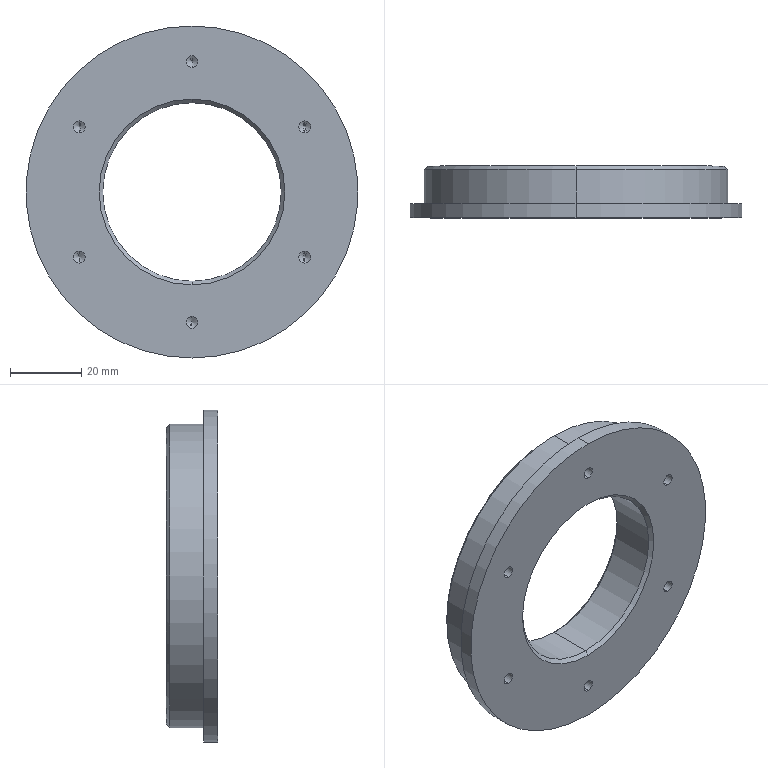Part | SolidWorks | features Chamfer 1, HoleWzd 1, Revolution 1 | 1 solid | 39 faces | box 93 x 14.5 x 93 mm | volume 57472 mm3 | cone 18 | cylinder 18 | plane 3 | commonest cylinder face diameters 3.3 x12 50 x2 85 x2 93 x2
STEP:
#1=CARTESIAN_POINT('',(0.,14.5,41.5));
#2=VERTEX_POINT('',#1);
#3=CARTESIAN_POINT('',(0.,14.5,-41.5));
#4=VERTEX_POINT('',#3);
#5=CARTESIAN_POINT('',(0.,14.5,0.));
#6=DIRECTION('',(0.,1.,0.));
#7=DIRECTION('',(0.,0.,1.));
#8=AXIS2_PLACEMENT_3D('',#5,#6,#7);
#9=CIRCLE('',#8,41.5);
#10=EDGE_CURVE('',#2,#4,#9,.T.);
#11=ORIENTED_EDGE('',*,*,#10,.F.);
#12=CARTESIAN_POINT('',(0.,13.5,42.5));
#13=VERTEX_POINT('',#12);
#14=CARTESIAN_POINT('',(0.,13.5,42.5));
#15=DIRECTION('',(0.,-0.7071,0.7071));
#16=VECTOR('',#15,1000.);
#17=LINE('',#14,#16);
#18=EDGE_CURVE('',#2,#13,#17,.T.);
#19=ORIENTED_EDGE('',*,*,#18,.T.);
#20=CARTESIAN_POINT('',(0.,13.5,-42.5));
#21=VERTEX_POINT('',#20);
#22=CARTESIAN_POINT('',(0.,13.5,0.));
#23=DIRECTION('',(0.,-1.,0.));
#24=DIRECTION('',(0.,0.,1.));
#25=AXIS2_PLACEMENT_3D('',#22,#23,#24);
#26=CIRCLE('',#25,42.5);
#27=EDGE_CURVE('',#21,#13,#26,.T.);
#28=ORIENTED_EDGE('',*,*,#27,.F.);
#29=CARTESIAN_POINT('',(0.,13.5,-42.5));
#30=DIRECTION('',(0.,-0.7071,-0.7071));
#31=VECTOR('',#30,1000.);
#32=LINE('',#29,#31);
#33=EDGE_CURVE('',#4,#21,#32,.T.);
#34=ORIENTED_EDGE('',*,*,#33,.F.);
#35=EDGE_LOOP('',(#11,#19,#28,#34));
#36=FACE_OUTER_BOUND('',#35,.T.);
#37=CARTESIAN_POINT('',(0.,13.5,0.));
#38=DIRECTION('',(0.,-1.,0.));
#39=DIRECTION('',(0.,0.,-1.));
#40=AXIS2_PLACEMENT_3D('',#37,#38,#39);
#41=CONICAL_SURFACE('',#40,42.5,0.7854);
#42=ADVANCED_FACE('',(#36),#41,.T.);
#43=CARTESIAN_POINT('',(0.,13.5,-25.));
#44=VERTEX_POINT('',#43);
#45=CARTESIAN_POINT('',(0.,13.5,25.));
#46=VERTEX_POINT('',#45);
#47=CARTESIAN_POINT('',(0.,13.5,0.));
#48=DIRECTION('',(0.,1.,0.));
#49=DIRECTION('',(0.,0.,1.));
#50=AXIS2_PLACEMENT_3D('',#47,#48,#49);
#51=CIRCLE('',#50,25.);
#52=EDGE_CURVE('',#44,#46,#51,.T.);
#53=ORIENTED_EDGE('',*,*,#52,.F.);
#54=CARTESIAN_POINT('',(0.,14.5,-26.));
#55=VERTEX_POINT('',#54);
#56=CARTESIAN_POINT('',(0.,14.5,-26.));
#57=DIRECTION('',(0.,0.7071,-0.7071));
#58=VECTOR('',#57,1000.);
#59=LINE('',#56,#58);
#60=EDGE_CURVE('',#44,#55,#59,.T.);
#61=ORIENTED_EDGE('',*,*,#60,.T.);
#62=CARTESIAN_POINT('',(0.,14.5,26.));
#63=VERTEX_POINT('',#62);
#64=CARTESIAN_POINT('',(0.,14.5,0.));
#65=DIRECTION('',(0.,-1.,0.));
#66=DIRECTION('',(0.,0.,1.));
#67=AXIS2_PLACEMENT_3D('',#64,#65,#66);
#68=CIRCLE('',#67,26.);
#69=EDGE_CURVE('',#63,#55,#68,.T.);
#70=ORIENTED_EDGE('',*,*,#69,.F.);
#71=CARTESIAN_POINT('',(0.,14.5,26.));
#72=DIRECTION('',(0.,0.7071,0.7071));
#73=VECTOR('',#72,1000.);
#74=LINE('',#71,#73);
#75=EDGE_CURVE('',#46,#63,#74,.T.);
#76=ORIENTED_EDGE('',*,*,#75,.F.);
#77=EDGE_LOOP('',(#53,#61,#70,#76));
#78=FACE_OUTER_BOUND('',#77,.T.);
#79=CARTESIAN_POINT('',(0.,14.5,0.));
#80=DIRECTION('',(0.,1.,0.));
#81=DIRECTION('',(0.,0.,1.));
#82=AXIS2_PLACEMENT_3D('',#79,#80,#81);
#83=CONICAL_SURFACE('',#82,26.,0.7854);
#84=ADVANCED_FACE('',(#78),#83,.F.);
#85=CARTESIAN_POINT('',(0.,1.,25.));
#86=VERTEX_POINT('',#85);
#87=CARTESIAN_POINT('',(0.,1.,-25.));
#88=VERTEX_POINT('',#87);
#89=CARTESIAN_POINT('',(0.,1.,0.));
#90=DIRECTION('',(0.,-1.,0.));
#91=DIRECTION('',(0.,0.,-1.));
#92=AXIS2_PLACEMENT_3D('',#89,#90,#91);
#93=CIRCLE('',#92,25.);
#94=EDGE_CURVE('',#86,#88,#93,.T.);
#95=ORIENTED_EDGE('',*,*,#94,.F.);
#96=CARTESIAN_POINT('',(0.,0.,26.));
#97=VERTEX_POINT('',#96);
#98=CARTESIAN_POINT('',(0.,1.,25.));
#99=DIRECTION('',(0.,-0.7071,0.7071));
#100=VECTOR('',#99,1000.);
#101=LINE('',#98,#100);
#102=EDGE_CURVE('',#86,#97,#101,.T.);
#103=ORIENTED_EDGE('',*,*,#102,.T.);
#104=CARTESIAN_POINT('',(0.,0.,-26.));
#105=VERTEX_POINT('',#104);
#106=CARTESIAN_POINT('',(0.,0.,0.));
#107=DIRECTION('',(0.,1.,0.));
#108=DIRECTION('',(0.,0.,-1.));
#109=AXIS2_PLACEMENT_3D('',#106,#107,#108);
#110=CIRCLE('',#109,26.);
#111=EDGE_CURVE('',#105,#97,#110,.T.);
#112=ORIENTED_EDGE('',*,*,#111,.F.);
#113=CARTESIAN_POINT('',(0.,1.,-25.));
#114=DIRECTION('',(0.,-0.7071,-0.7071));
#115=VECTOR('',#114,1000.);
#116=LINE('',#113,#115);
#117=EDGE_CURVE('',#88,#105,#116,.T.);
#118=ORIENTED_EDGE('',*,*,#117,.F.);
#119=EDGE_LOOP('',(#95,#103,#112,#118));
#120=FACE_OUTER_BOUND('',#119,.T.);
#121=CARTESIAN_POINT('',(0.,1.,0.));
#122=DIRECTION('',(0.,-1.,0.));
#123=DIRECTION('',(0.,0.,-1.));
#124=AXIS2_PLACEMENT_3D('',#121,#122,#123);
#125=CONICAL_SURFACE('',#124,25.,0.7854);
#126=ADVANCED_FACE('',(#120),#125,.F.);
#127=CARTESIAN_POINT('',(0.,9.8,38.15));
#128=VERTEX_POINT('',#127);
#129=CARTESIAN_POINT('',(0.,9.8,34.85));
#130=VERTEX_POINT('',#129);
#131=CARTESIAN_POINT('',(0.,9.8,36.5));
#132=DIRECTION('',(0.,-1.,0.));
#133=DIRECTION('',(0.,0.,-1.));
#134=AXIS2_PLACEMENT_3D('',#131,#132,#133);
#135=CIRCLE('',#134,1.65);
#136=EDGE_CURVE('',#128,#130,#135,.T.);
#137=ORIENTED_EDGE('',*,*,#136,.F.);
#138=CARTESIAN_POINT('',(0.,0.,38.15));
#139=VERTEX_POINT('',#138);
#140=CARTESIAN_POINT('',(0.,0.,38.15));
#141=DIRECTION('',(0.,-1.,0.));
#142=VECTOR('',#141,1000.);
#143=LINE('',#140,#142);
#144=EDGE_CURVE('',#128,#139,#143,.T.);
#145=ORIENTED_EDGE('',*,*,#144,.T.);
#146=CARTESIAN_POINT('',(0.,0.,34.85));
#147=VERTEX_POINT('',#146);
#148=CARTESIAN_POINT('',(0.,0.,36.5));
#149=DIRECTION('',(0.,-1.,0.));
#150=DIRECTION('',(0.,0.,-1.));
#151=AXIS2_PLACEMENT_3D('',#148,#149,#150);
#152=CIRCLE('',#151,1.65);
#153=EDGE_CURVE('',#139,#147,#152,.T.);
#154=ORIENTED_EDGE('',*,*,#153,.T.);
#155=CARTESIAN_POINT('',(0.,0.,34.85));
#156=DIRECTION('',(0.,-1.,0.));
#157=VECTOR('',#156,1000.);
#158=LINE('',#155,#157);
#159=EDGE_CURVE('',#130,#147,#158,.T.);
#160=ORIENTED_EDGE('',*,*,#159,.F.);
#161=EDGE_LOOP('',(#137,#145,#154,#160));
#162=FACE_OUTER_BOUND('',#161,.T.);
#163=CARTESIAN_POINT('',(0.,0.,36.5));
#164=DIRECTION('',(0.,-1.,0.));
#165=DIRECTION('',(0.,0.,-1.));
#166=AXIS2_PLACEMENT_3D('',#163,#164,#165);
#167=CYLINDRICAL_SURFACE('',#166,1.65);
#168=ADVANCED_FACE('',(#162),#167,.F.);
#169=CARTESIAN_POINT('',(0.,10.791,36.5));
#170=VERTEX_POINT('',#169);
#171=CARTESIAN_POINT('',(0.,9.8,34.85));
#172=DIRECTION('',(0.,-0.515,-0.8572));
#173=VECTOR('',#172,1000.);
#174=LINE('',#171,#173);
#175=EDGE_CURVE('',#170,#130,#174,.T.);
#176=ORIENTED_EDGE('',*,*,#175,.F.);
#177=CARTESIAN_POINT('',(0.,9.8,38.15));
#178=DIRECTION('',(0.,-0.515,0.8572));
#179=VECTOR('',#178,1000.);
#180=LINE('',#177,#179);
#181=EDGE_CURVE('',#170,#128,#180,.T.);
#182=ORIENTED_EDGE('',*,*,#181,.T.);
#183=ORIENTED_EDGE('',*,*,#136,.T.);
#184=EDGE_LOOP('',(#176,#182,#183));
#185=FACE_OUTER_BOUND('',#184,.T.);
#186=CARTESIAN_POINT('',(0.,9.8,36.5));
#187=DIRECTION('',(0.,-1.,0.));
#188=DIRECTION('',(0.,0.,-1.));
#189=AXIS2_PLACEMENT_3D('',#186,#187,#188);
#190=CONICAL_SURFACE('',#189,1.65,1.03);
#191=ADVANCED_FACE('',(#185),#190,.F.);
#192=CARTESIAN_POINT('',(31.61,9.8,19.9));
#193=VERTEX_POINT('',#192);
#194=CARTESIAN_POINT('',(31.61,9.8,16.6));
#195=VERTEX_POINT('',#194);
#196=CARTESIAN_POINT('',(31.61,9.8,18.25));
#197=DIRECTION('',(0.,-1.,0.));
#198=DIRECTION('',(0.,0.,-1.));
#199=AXIS2_PLACEMENT_3D('',#196,#197,#198);
#200=CIRCLE('',#199,1.65);
#201=EDGE_CURVE('',#193,#195,#200,.T.);
#202=ORIENTED_EDGE('',*,*,#201,.F.);
#203=CARTESIAN_POINT('',(31.61,0.,19.9));
#204=VERTEX_POINT('',#203);
#205=CARTESIAN_POINT('',(31.61,0.,19.9));
#206=DIRECTION('',(0.,-1.,0.));
#207=VECTOR('',#206,1000.);
#208=LINE('',#205,#207);
#209=EDGE_CURVE('',#193,#204,#208,.T.);
#210=ORIENTED_EDGE('',*,*,#209,.T.);
#211=CARTESIAN_POINT('',(31.61,0.,16.6));
#212=VERTEX_POINT('',#211);
#213=CARTESIAN_POINT('',(31.61,0.,18.25));
#214=DIRECTION('',(0.,-1.,0.));
#215=DIRECTION('',(0.,0.,-1.));
#216=AXIS2_PLACEMENT_3D('',#213,#214,#215);
#217=CIRCLE('',#216,1.65);
#218=EDGE_CURVE('',#204,#212,#217,.T.);
#219=ORIENTED_EDGE('',*,*,#218,.T.);
#220=CARTESIAN_POINT('',(31.61,0.,16.6));
#221=DIRECTION('',(0.,-1.,0.));
#222=VECTOR('',#221,1000.);
#223=LINE('',#220,#222);
#224=EDGE_CURVE('',#195,#212,#223,.T.);
#225=ORIENTED_EDGE('',*,*,#224,.F.);
#226=EDGE_LOOP('',(#202,#210,#219,#225));
#227=FACE_OUTER_BOUND('',#226,.T.);
#228=CARTESIAN_POINT('',(31.61,0.,18.25));
#229=DIRECTION('',(0.,-1.,0.));
#230=DIRECTION('',(0.,0.,-1.));
#231=AXIS2_PLACEMENT_3D('',#228,#229,#230);
#232=CYLINDRICAL_SURFACE('',#231,1.65);
#233=ADVANCED_FACE('',(#227),#232,.F.);
#234=CARTESIAN_POINT('',(31.61,10.791,18.25));
#235=VERTEX_POINT('',#234);
#236=CARTESIAN_POINT('',(31.61,9.8,16.6));
#237=DIRECTION('',(0.,-0.515,-0.8572));
#238=VECTOR('',#237,1000.);
#239=LINE('',#236,#238);
#240=EDGE_CURVE('',#235,#195,#239,.T.);
#241=ORIENTED_EDGE('',*,*,#240,.F.);
#242=CARTESIAN_POINT('',(31.61,9.8,19.9));
#243=DIRECTION('',(0.,-0.515,0.8572));
#244=VECTOR('',#243,1000.);
#245=LINE('',#242,#244);
#246=EDGE_CURVE('',#235,#193,#245,.T.);
#247=ORIENTED_EDGE('',*,*,#246,.T.);
#248=ORIENTED_EDGE('',*,*,#201,.T.);
#249=EDGE_LOOP('',(#241,#247,#248));
#250=FACE_OUTER_BOUND('',#249,.T.);
#251=CARTESIAN_POINT('',(31.61,9.8,18.25));
#252=DIRECTION('',(0.,-1.,0.));
#253=DIRECTION('',(0.,0.,-1.));
#254=AXIS2_PLACEMENT_3D('',#251,#252,#253);
#255=CONICAL_SURFACE('',#254,1.65,1.03);
#256=ADVANCED_FACE('',(#250),#255,.F.);
#257=CARTESIAN_POINT('',(31.61,9.8,-16.6));
#258=VERTEX_POINT('',#257);
#259=CARTESIAN_POINT('',(31.61,9.8,-19.9));
#260=VERTEX_POINT('',#259);
#261=CARTESIAN_POINT('',(31.61,9.8,-18.25));
#262=DIRECTION('',(0.,-1.,0.));
#263=DIRECTION('',(0.,0.,-1.));
#264=AXIS2_PLACEMENT_3D('',#261,#262,#263);
#265=CIRCLE('',#264,1.65);
#266=EDGE_CURVE('',#258,#260,#265,.T.);
#267=ORIENTED_EDGE('',*,*,#266,.F.);
#268=CARTESIAN_POINT('',(31.61,0.,-16.6));
#269=VERTEX_POINT('',#268);
#270=CARTESIAN_POINT('',(31.61,0.,-16.6));
#271=DIRECTION('',(0.,-1.,0.));
#272=VECTOR('',#271,1000.);
#273=LINE('',#270,#272);
#274=EDGE_CURVE('',#258,#269,#273,.T.);
#275=ORIENTED_EDGE('',*,*,#274,.T.);
#276=CARTESIAN_POINT('',(31.61,0.,-19.9));
#277=VERTEX_POINT('',#276);
#278=CARTESIAN_POINT('',(31.61,0.,-18.25));
#279=DIRECTION('',(0.,-1.,0.));
#280=DIRECTION('',(0.,0.,-1.));
#281=AXIS2_PLACEMENT_3D('',#278,#279,#280);
#282=CIRCLE('',#281,1.65);
#283=EDGE_CURVE('',#269,#277,#282,.T.);
#284=ORIENTED_EDGE('',*,*,#283,.T.);
#285=CARTESIAN_POINT('',(31.61,0.,-19.9));
#286=DIRECTION('',(0.,-1.,0.));
#287=VECTOR('',#286,1000.);
#288=LINE('',#285,#287);
#289=EDGE_CURVE('',#260,#277,#288,.T.);
#290=ORIENTED_EDGE('',*,*,#289,.F.);
#291=EDGE_LOOP('',(#267,#275,#284,#290));
#292=FACE_OUTER_BOUND('',#291,.T.);
#293=CARTESIAN_POINT('',(31.61,0.,-18.25));
#294=DIRECTION('',(0.,-1.,0.));
#295=DIRECTION('',(0.,0.,-1.));
#296=AXIS2_PLACEMENT_3D('',#293,#294,#295);
#297=CYLINDRICAL_SURFACE('',#296,1.65);
#298=ADVANCED_FACE('',(#292),#297,.F.);
#299=CARTESIAN_POINT('',(31.61,10.791,-18.25));
#300=VERTEX_POINT('',#299);
#301=CARTESIAN_POINT('',(31.61,9.8,-19.9));
#302=DIRECTION('',(0.,-0.515,-0.8572));
#303=VECTOR('',#302,1000.);
#304=LINE('',#301,#303);
#305=EDGE_CURVE('',#300,#260,#304,.T.);
#306=ORIENTED_EDGE('',*,*,#305,.F.);
#307=CARTESIAN_POINT('',(31.61,9.8,-16.6));
#308=DIRECTION('',(0.,-0.515,0.8572));
#309=VECTOR('',#308,1000.);
#310=LINE('',#307,#309);
#311=EDGE_CURVE('',#300,#258,#310,.T.);
#312=ORIENTED_EDGE('',*,*,#311,.T.);
#313=ORIENTED_EDGE('',*,*,#266,.T.);
#314=EDGE_LOOP('',(#306,#312,#313));
#315=FACE_OUTER_BOUND('',#314,.T.);
#316=CARTESIAN_POINT('',(31.61,9.8,-18.25));
#317=DIRECTION('',(0.,-1.,0.));
#318=DIRECTION('',(0.,0.,-1.));
#319=AXIS2_PLACEMENT_3D('',#316,#317,#318);
#320=CONICAL_SURFACE('',#319,1.65,1.03);
#321=ADVANCED_FACE('',(#315),#320,.F.);
#322=CARTESIAN_POINT('',(0.,9.8,-34.85));
#323=VERTEX_POINT('',#322);
#324=CARTESIAN_POINT('',(0.,9.8,-38.15));
#325=VERTEX_POINT('',#324);
#326=CARTESIAN_POINT('',(0.,9.8,-36.5));
#327=DIRECTION('',(0.,-1.,0.));
#328=DIRECTION('',(0.,0.,-1.));
#329=AXIS2_PLACEMENT_3D('',#326,#327,#328);
#330=CIRCLE('',#329,1.65);
#331=EDGE_CURVE('',#323,#325,#330,.T.);
#332=ORIENTED_EDGE('',*,*,#331,.F.);
#333=CARTESIAN_POINT('',(0.,0.,-34.85));
#334=VERTEX_POINT('',#333);
#335=CARTESIAN_POINT('',(0.,0.,-34.85));
#336=DIRECTION('',(0.,-1.,0.));
#337=VECTOR('',#336,1000.);
#338=LINE('',#335,#337);
#339=EDGE_CURVE('',#323,#334,#338,.T.);
#340=ORIENTED_EDGE('',*,*,#339,.T.);
#341=CARTESIAN_POINT('',(0.,0.,-38.15));
#342=VERTEX_POINT('',#341);
#343=CARTESIAN_POINT('',(0.,0.,-36.5));
#344=DIRECTION('',(0.,-1.,0.));
#345=DIRECTION('',(0.,0.,-1.));
#346=AXIS2_PLACEMENT_3D('',#343,#344,#345);
#347=CIRCLE('',#346,1.65);
#348=EDGE_CURVE('',#334,#342,#347,.T.);
#349=ORIENTED_EDGE('',*,*,#348,.T.);
#350=CARTESIAN_POINT('',(0.,0.,-38.15));
#351=DIRECTION('',(0.,-1.,0.));
#352=VECTOR('',#351,1000.);
#353=LINE('',#350,#352);
#354=EDGE_CURVE('',#325,#342,#353,.T.);
#355=ORIENTED_EDGE('',*,*,#354,.F.);
#356=EDGE_LOOP('',(#332,#340,#349,#355));
#357=FACE_OUTER_BOUND('',#356,.T.);
#358=CARTESIAN_POINT('',(0.,0.,-36.5));
#359=DIRECTION('',(0.,-1.,0.));
#360=DIRECTION('',(0.,0.,-1.));
#361=AXIS2_PLACEMENT_3D('',#358,#359,#360);
#362=CYLINDRICAL_SURFACE('',#361,1.65);
#363=ADVANCED_FACE('',(#357),#362,.F.);
#364=CARTESIAN_POINT('',(0.,10.791,-36.5));
#365=VERTEX_POINT('',#364);
#366=CARTESIAN_POINT('',(0.,9.8,-38.15));
#367=DIRECTION('',(0.,-0.515,-0.8572));
#368=VECTOR('',#367,1000.);
#369=LINE('',#366,#368);
#370=EDGE_CURVE('',#365,#325,#369,.T.);
#371=ORIENTED_EDGE('',*,*,#370,.F.);
#372=CARTESIAN_POINT('',(0.,9.8,-34.85));
#373=DIRECTION('',(0.,-0.515,0.8572));
#374=VECTOR('',#373,1000.);
#375=LINE('',#372,#374);
#376=EDGE_CURVE('',#365,#323,#375,.T.);
#377=ORIENTED_EDGE('',*,*,#376,.T.);
#378=ORIENTED_EDGE('',*,*,#331,.T.);
#379=EDGE_LOOP('',(#371,#377,#378));
#380=FACE_OUTER_BOUND('',#379,.T.);
#381=CARTESIAN_POINT('',(0.,9.8,-36.5));
#382=DIRECTION('',(0.,-1.,0.));
#383=DIRECTION('',(0.,0.,-1.));
#384=AXIS2_PLACEMENT_3D('',#381,#382,#383);
#385=CONICAL_SURFACE('',#384,1.65,1.03);
#386=ADVANCED_FACE('',(#380),#385,.F.);
#387=CARTESIAN_POINT('',(-31.61,9.8,-16.6));
#388=VERTEX_POINT('',#387);
#389=CARTESIAN_POINT('',(-31.61,9.8,-19.9));
#390=VERTEX_POINT('',#389);
#391=CARTESIAN_POINT('',(-31.61,9.8,-18.25));
#392=DIRECTION('',(0.,-1.,0.));
#393=DIRECTION('',(0.,0.,-1.));
#394=AXIS2_PLACEMENT_3D('',#391,#392,#393);
#395=CIRCLE('',#394,1.65);
#396=EDGE_CURVE('',#388,#390,#395,.T.);
#397=ORIENTED_EDGE('',*,*,#396,.F.);
#398=CARTESIAN_POINT('',(-31.61,0.,-16.6));
#399=VERTEX_POINT('',#398);
#400=CARTESIAN_POINT('',(-31.61,0.,-16.6));
#401=DIRECTION('',(0.,-1.,0.));
#402=VECTOR('',#401,1000.);
#403=LINE('',#400,#402);
#404=EDGE_CURVE('',#388,#399,#403,.T.);
#405=ORIENTED_EDGE('',*,*,#404,.T.);
#406=CARTESIAN_POINT('',(-31.61,0.,-19.9));
#407=VERTEX_POINT('',#406);
#408=CARTESIAN_POINT('',(-31.61,0.,-18.25));
#409=DIRECTION('',(0.,-1.,0.));
#410=DIRECTION('',(0.,0.,-1.));
#411=AXIS2_PLACEMENT_3D('',#408,#409,#410);
#412=CIRCLE('',#411,1.65);
#413=EDGE_CURVE('',#399,#407,#412,.T.);
#414=ORIENTED_EDGE('',*,*,#413,.T.);
#415=CARTESIAN_POINT('',(-31.61,0.,-19.9));
#416=DIRECTION('',(0.,-1.,0.));
#417=VECTOR('',#416,1000.);
#418=LINE('',#415,#417);
#419=EDGE_CURVE('',#390,#407,#418,.T.);
#420=ORIENTED_EDGE('',*,*,#419,.F.);
#421=EDGE_LOOP('',(#397,#405,#414,#420));
#422=FACE_OUTER_BOUND('',#421,.T.);
#423=CARTESIAN_POINT('',(-31.61,0.,-18.25));
#424=DIRECTION('',(0.,-1.,0.));
#425=DIRECTION('',(0.,0.,-1.));
#426=AXIS2_PLACEMENT_3D('',#423,#424,#425);
#427=CYLINDRICAL_SURFACE('',#426,1.65);
#428=ADVANCED_FACE('',(#422),#427,.F.);
#429=CARTESIAN_POINT('',(-31.61,10.791,-18.25));
#430=VERTEX_POINT('',#429);
#431=CARTESIAN_POINT('',(-31.61,9.8,-19.9));
#432=DIRECTION('',(0.,-0.515,-0.8572));
#433=VECTOR('',#432,1000.);
#434=LINE('',#431,#433);
#435=EDGE_CURVE('',#430,#390,#434,.T.);
#436=ORIENTED_EDGE('',*,*,#435,.F.);
#437=CARTESIAN_POINT('',(-31.61,9.8,-16.6));
#438=DIRECTION('',(0.,-0.515,0.8572));
#439=VECTOR('',#438,1000.);
#440=LINE('',#437,#439);
#441=EDGE_CURVE('',#430,#388,#440,.T.);
#442=ORIENTED_EDGE('',*,*,#441,.T.);
#443=ORIENTED_EDGE('',*,*,#396,.T.);
#444=EDGE_LOOP('',(#436,#442,#443));
#445=FACE_OUTER_BOUND('',#444,.T.);
#446=CARTESIAN_POINT('',(-31.61,9.8,-18.25));
#447=DIRECTION('',(0.,-1.,0.));
#448=DIRECTION('',(0.,0.,-1.));
#449=AXIS2_PLACEMENT_3D('',#446,#447,#448);
#450=CONICAL_SURFACE('',#449,1.65,1.03);
#451=ADVANCED_FACE('',(#445),#450,.F.);
#452=CARTESIAN_POINT('',(-31.61,9.8,19.9));
#453=VERTEX_POINT('',#452);
#454=CARTESIAN_POINT('',(-31.61,9.8,16.6));
#455=VERTEX_POINT('',#454);
#456=CARTESIAN_POINT('',(-31.61,9.8,18.25));
#457=DIRECTION('',(0.,-1.,0.));
#458=DIRECTION('',(0.,0.,-1.));
#459=AXIS2_PLACEMENT_3D('',#456,#457,#458);
#460=CIRCLE('',#459,1.65);
#461=EDGE_CURVE('',#453,#455,#460,.T.);
#462=ORIENTED_EDGE('',*,*,#461,.F.);
#463=CARTESIAN_POINT('',(-31.61,0.,19.9));
#464=VERTEX_POINT('',#463);
#465=CARTESIAN_POINT('',(-31.61,0.,19.9));
#466=DIRECTION('',(0.,-1.,0.));
#467=VECTOR('',#466,1000.);
#468=LINE('',#465,#467);
#469=EDGE_CURVE('',#453,#464,#468,.T.);
#470=ORIENTED_EDGE('',*,*,#469,.T.);
#471=CARTESIAN_POINT('',(-31.61,0.,16.6));
#472=VERTEX_POINT('',#471);
#473=CARTESIAN_POINT('',(-31.61,0.,18.25));
#474=DIRECTION('',(0.,-1.,0.));
#475=DIRECTION('',(0.,0.,-1.));
#476=AXIS2_PLACEMENT_3D('',#473,#474,#475);
#477=CIRCLE('',#476,1.65);
#478=EDGE_CURVE('',#464,#472,#477,.T.);
#479=ORIENTED_EDGE('',*,*,#478,.T.);
#480=CARTESIAN_POINT('',(-31.61,0.,16.6));
#481=DIRECTION('',(0.,-1.,0.));
#482=VECTOR('',#481,1000.);
#483=LINE('',#480,#482);
#484=EDGE_CURVE('',#455,#472,#483,.T.);
#485=ORIENTED_EDGE('',*,*,#484,.F.);
#486=EDGE_LOOP('',(#462,#470,#479,#485));
#487=FACE_OUTER_BOUND('',#486,.T.);
#488=CARTESIAN_POINT('',(-31.61,0.,18.25));
#489=DIRECTION('',(0.,-1.,0.));
#490=DIRECTION('',(0.,0.,-1.));
#491=AXIS2_PLACEMENT_3D('',#488,#489,#490);
#492=CYLINDRICAL_SURFACE('',#491,1.65);
#493=ADVANCED_FACE('',(#487),#492,.F.);
#494=CARTESIAN_POINT('',(-31.61,10.791,18.25));
#495=VERTEX_POINT('',#494);
#496=CARTESIAN_POINT('',(-31.61,9.8,16.6));
#497=DIRECTION('',(0.,-0.515,-0.8572));
#498=VECTOR('',#497,1000.);
#499=LINE('',#496,#498);
#500=EDGE_CURVE('',#495,#455,#499,.T.);
#501=ORIENTED_EDGE('',*,*,#500,.F.);
#502=CARTESIAN_POINT('',(-31.61,9.8,19.9));
#503=DIRECTION('',(0.,-0.515,0.8572));
#504=VECTOR('',#503,1000.);
#505=LINE('',#502,#504);
#506=EDGE_CURVE('',#495,#453,#505,.T.);
#507=ORIENTED_EDGE('',*,*,#506,.T.);
#508=ORIENTED_EDGE('',*,*,#461,.T.);
#509=EDGE_LOOP('',(#501,#507,#508));
#510=FACE_OUTER_BOUND('',#509,.T.);
#511=CARTESIAN_POINT('',(-31.61,9.8,18.25));
#512=DIRECTION('',(0.,-1.,0.));
#513=DIRECTION('',(0.,0.,-1.));
#514=AXIS2_PLACEMENT_3D('',#511,#512,#513);
#515=CONICAL_SURFACE('',#514,1.65,1.03);
#516=ADVANCED_FACE('',(#510),#515,.F.);
#517=ORIENTED_EDGE('',*,*,#52,.T.);
#518=CARTESIAN_POINT('',(0.,0.,25.));
#519=DIRECTION('',(0.,-1.,0.));
#520=VECTOR('',#519,1000.);
#521=LINE('',#518,#520);
#522=EDGE_CURVE('',#46,#86,#521,.T.);
#523=ORIENTED_EDGE('',*,*,#522,.T.);
#524=ORIENTED_EDGE('',*,*,#94,.T.);
#525=CARTESIAN_POINT('',(0.,0.,-25.));
#526=DIRECTION('',(0.,-1.,0.));
#527=VECTOR('',#526,1000.);
#528=LINE('',#525,#527);
#529=EDGE_CURVE('',#44,#88,#528,.T.);
#530=ORIENTED_EDGE('',*,*,#529,.F.);
#531=EDGE_LOOP('',(#517,#523,#524,#530));
#532=FACE_OUTER_BOUND('',#531,.T.);
#533=CARTESIAN_POINT('',(0.,0.,0.));
#534=DIRECTION('',(0.,-1.,0.));
#535=DIRECTION('',(0.,0.,-1.));
#536=AXIS2_PLACEMENT_3D('',#533,#534,#535);
#537=CYLINDRICAL_SURFACE('',#536,25.);
#538=ADVANCED_FACE('',(#532),#537,.F.);
#539=ORIENTED_EDGE('',*,*,#27,.T.);
#540=CARTESIAN_POINT('',(0.,4.,42.5));
#541=VERTEX_POINT('',#540);
#542=CARTESIAN_POINT('',(0.,0.,42.5));
#543=DIRECTION('',(0.,-1.,0.));
#544=VECTOR('',#543,1000.);
#545=LINE('',#542,#544);
#546=EDGE_CURVE('',#13,#541,#545,.T.);
#547=ORIENTED_EDGE('',*,*,#546,.T.);
#548=CARTESIAN_POINT('',(0.,4.,-42.5));
#549=VERTEX_POINT('',#548);
#550=CARTESIAN_POINT('',(0.,4.,0.));
#551=DIRECTION('',(0.,-1.,0.));
#552=DIRECTION('',(0.,0.,-1.));
#553=AXIS2_PLACEMENT_3D('',#550,#551,#552);
#554=CIRCLE('',#553,42.5);
#555=EDGE_CURVE('',#549,#541,#554,.T.);
#556=ORIENTED_EDGE('',*,*,#555,.F.);
#557=CARTESIAN_POINT('',(0.,0.,-42.5));
#558=DIRECTION('',(0.,-1.,0.));
#559=VECTOR('',#558,1000.);
#560=LINE('',#557,#559);
#561=EDGE_CURVE('',#21,#549,#560,.T.);
#562=ORIENTED_EDGE('',*,*,#561,.F.);
#563=EDGE_LOOP('',(#539,#547,#556,#562));
#564=FACE_OUTER_BOUND('',#563,.T.);
#565=CARTESIAN_POINT('',(0.,0.,0.));
#566=DIRECTION('',(0.,-1.,0.));
#567=DIRECTION('',(0.,0.,-1.));
#568=AXIS2_PLACEMENT_3D('',#565,#566,#567);
#569=CYLINDRICAL_SURFACE('',#568,42.5);
#570=ADVANCED_FACE('',(#564),#569,.T.);
#571=CARTESIAN_POINT('',(0.,4.,-46.5));
#572=VERTEX_POINT('',#571);
#573=CARTESIAN_POINT('',(0.,4.,46.5));
#574=VERTEX_POINT('',#573);
#575=CARTESIAN_POINT('',(0.,4.,0.));
#576=DIRECTION('',(0.,-1.,0.));
#577=DIRECTION('',(0.,0.,-1.));
#578=AXIS2_PLACEMENT_3D('',#575,#576,#577);
#579=CIRCLE('',#578,46.5);
#580=EDGE_CURVE('',#572,#574,#579,.T.);
#581=ORIENTED_EDGE('',*,*,#580,.T.);
#582=CARTESIAN_POINT('',(0.,0.,46.5));
#583=VERTEX_POINT('',#582);
#584=CARTESIAN_POINT('',(0.,0.,46.5));
#585=DIRECTION('',(0.,-1.,0.));
#586=VECTOR('',#585,1000.);
#587=LINE('',#584,#586);
#588=EDGE_CURVE('',#574,#583,#587,.T.);
#589=ORIENTED_EDGE('',*,*,#588,.T.);
#590=CARTESIAN_POINT('',(0.,0.,-46.5));
#591=VERTEX_POINT('',#590);
#592=CARTESIAN_POINT('',(0.,0.,0.));
#593=DIRECTION('',(0.,-1.,0.));
#594=DIRECTION('',(0.,0.,-1.));
#595=AXIS2_PLACEMENT_3D('',#592,#593,#594);
#596=CIRCLE('',#595,46.5);
#597=EDGE_CURVE('',#591,#583,#596,.T.);
#598=ORIENTED_EDGE('',*,*,#597,.F.);
#599=CARTESIAN_POINT('',(0.,0.,-46.5));
#600=DIRECTION('',(0.,-1.,0.));
#601=VECTOR('',#600,1000.);
#602=LINE('',#599,#601);
#603=EDGE_CURVE('',#572,#591,#602,.T.);
#604=ORIENTED_EDGE('',*,*,#603,.F.);
#605=EDGE_LOOP('',(#581,#589,#598,#604));
#606=FACE_OUTER_BOUND('',#605,.T.);
#607=CARTESIAN_POINT('',(0.,0.,0.));
#608=DIRECTION('',(0.,-1.,0.));
#609=DIRECTION('',(0.,0.,-1.));
#610=AXIS2_PLACEMENT_3D('',#607,#608,#609);
#611=CYLINDRICAL_SURFACE('',#610,46.5);
#612=ADVANCED_FACE('',(#606),#611,.T.);
#613=ORIENTED_EDGE('',*,*,#588,.F.);
#614=CARTESIAN_POINT('',(0.,4.,0.));
#615=DIRECTION('',(0.,-1.,0.));
#616=DIRECTION('',(0.,0.,-1.));
#617=AXIS2_PLACEMENT_3D('',#614,#615,#616);
#618=CIRCLE('',#617,46.5);
#619=EDGE_CURVE('',#574,#572,#618,.T.);
#620=ORIENTED_EDGE('',*,*,#619,.T.);
#621=ORIENTED_EDGE('',*,*,#603,.T.);
#622=CARTESIAN_POINT('',(0.,0.,0.));
#623=DIRECTION('',(0.,-1.,0.));
#624=DIRECTION('',(0.,0.,-1.));
#625=AXIS2_PLACEMENT_3D('',#622,#623,#624);
#626=CIRCLE('',#625,46.5);
#627=EDGE_CURVE('',#583,#591,#626,.T.);
#628=ORIENTED_EDGE('',*,*,#627,.F.);
#629=EDGE_LOOP('',(#613,#620,#621,#628));
#630=FACE_OUTER_BOUND('',#629,.T.);
#631=CARTESIAN_POINT('',(0.,0.,0.));
#632=DIRECTION('',(0.,-1.,0.));
#633=DIRECTION('',(0.,0.,-1.));
#634=AXIS2_PLACEMENT_3D('',#631,#632,#633);
#635=CYLINDRICAL_SURFACE('',#634,46.5);
#636=ADVANCED_FACE('',(#630),#635,.T.);
#637=ORIENTED_EDGE('',*,*,#555,.T.);
#638=CARTESIAN_POINT('',(0.,4.,0.));
#639=DIRECTION('',(0.,-1.,0.));
#640=DIRECTION('',(0.,0.,-1.));
#641=AXIS2_PLACEMENT_3D('',#638,#639,#640);
#642=CIRCLE('',#641,42.5);
#643=EDGE_CURVE('',#541,#549,#642,.T.);
#644=ORIENTED_EDGE('',*,*,#643,.T.);
#645=EDGE_LOOP('',(#637,#644));
#646=FACE_BOUND('',#645,.T.);
#647=ORIENTED_EDGE('',*,*,#580,.F.);
#648=ORIENTED_EDGE('',*,*,#619,.F.);
#649=EDGE_LOOP('',(#647,#648));
#650=FACE_OUTER_BOUND('',#649,.T.);
#651=CARTESIAN_POINT('',(46.5,4.,0.));
#652=DIRECTION('',(0.,1.,0.));
#653=DIRECTION('',(0.,0.,1.));
#654=AXIS2_PLACEMENT_3D('',#651,#652,#653);
#655=PLANE('',#654);
#656=ADVANCED_FACE('',(#646,#650),#655,.T.);
#657=ORIENTED_EDGE('',*,*,#546,.F.);
#658=CARTESIAN_POINT('',(0.,13.5,0.));
#659=DIRECTION('',(0.,-1.,0.));
#660=DIRECTION('',(0.,0.,1.));
#661=AXIS2_PLACEMENT_3D('',#658,#659,#660);
#662=CIRCLE('',#661,42.5);
#663=EDGE_CURVE('',#13,#21,#662,.T.);
#664=ORIENTED_EDGE('',*,*,#663,.T.);
#665=ORIENTED_EDGE('',*,*,#561,.T.);
#666=ORIENTED_EDGE('',*,*,#643,.F.);
#667=EDGE_LOOP('',(#657,#664,#665,#666));
#668=FACE_OUTER_BOUND('',#667,.T.);
#669=CARTESIAN_POINT('',(0.,0.,0.));
#670=DIRECTION('',(0.,-1.,0.));
#671=DIRECTION('',(0.,0.,-1.));
#672=AXIS2_PLACEMENT_3D('',#669,#670,#671);
#673=CYLINDRICAL_SURFACE('',#672,42.5);
#674=ADVANCED_FACE('',(#668),#673,.T.);
#675=ORIENTED_EDGE('',*,*,#69,.T.);
#676=CARTESIAN_POINT('',(0.,14.5,0.));
#677=DIRECTION('',(0.,-1.,0.));
#678=DIRECTION('',(0.,0.,1.));
#679=AXIS2_PLACEMENT_3D('',#676,#677,#678);
#680=CIRCLE('',#679,26.);
#681=EDGE_CURVE('',#55,#63,#680,.T.);
#682=ORIENTED_EDGE('',*,*,#681,.T.);
#683=EDGE_LOOP('',(#675,#682));
#684=FACE_BOUND('',#683,.T.);
#685=CARTESIAN_POINT('',(0.,14.5,0.));
#686=DIRECTION('',(0.,1.,0.));
#687=DIRECTION('',(0.,0.,1.));
#688=AXIS2_PLACEMENT_3D('',#685,#686,#687);
#689=CIRCLE('',#688,41.5);
#690=EDGE_CURVE('',#4,#2,#689,.T.);
#691=ORIENTED_EDGE('',*,*,#690,.T.);
#692=ORIENTED_EDGE('',*,*,#10,.T.);
#693=EDGE_LOOP('',(#691,#692));
#694=FACE_OUTER_BOUND('',#693,.T.);
#695=CARTESIAN_POINT('',(42.5,14.5,0.));
#696=DIRECTION('',(0.,1.,0.));
#697=DIRECTION('',(0.,0.,1.));
#698=AXIS2_PLACEMENT_3D('',#695,#696,#697);
#699=PLANE('',#698);
#700=ADVANCED_FACE('',(#684,#694),#699,.T.);
#701=ORIENTED_EDGE('',*,*,#522,.F.);
#702=CARTESIAN_POINT('',(0.,13.5,0.));
#703=DIRECTION('',(0.,1.,0.));
#704=DIRECTION('',(0.,0.,1.));
#705=AXIS2_PLACEMENT_3D('',#702,#703,#704);
#706=CIRCLE('',#705,25.);
#707=EDGE_CURVE('',#46,#44,#706,.T.);
#708=ORIENTED_EDGE('',*,*,#707,.T.);
#709=ORIENTED_EDGE('',*,*,#529,.T.);
#710=CARTESIAN_POINT('',(0.,1.,0.));
#711=DIRECTION('',(0.,-1.,0.));
#712=DIRECTION('',(0.,0.,-1.));
#713=AXIS2_PLACEMENT_3D('',#710,#711,#712);
#714=CIRCLE('',#713,25.);
#715=EDGE_CURVE('',#88,#86,#714,.T.);
#716=ORIENTED_EDGE('',*,*,#715,.T.);
#717=EDGE_LOOP('',(#701,#708,#709,#716));
#718=FACE_OUTER_BOUND('',#717,.T.);
#719=CARTESIAN_POINT('',(0.,0.,0.));
#720=DIRECTION('',(0.,-1.,0.));
#721=DIRECTION('',(0.,0.,-1.));
#722=AXIS2_PLACEMENT_3D('',#719,#720,#721);
#723=CYLINDRICAL_SURFACE('',#722,25.);
#724=ADVANCED_FACE('',(#718),#723,.F.);
#725=ORIENTED_EDGE('',*,*,#111,.T.);
#726=CARTESIAN_POINT('',(0.,0.,0.));
#727=DIRECTION('',(0.,1.,0.));
#728=DIRECTION('',(0.,0.,-1.));
#729=AXIS2_PLACEMENT_3D('',#726,#727,#728);
#730=CIRCLE('',#729,26.);
#731=EDGE_CURVE('',#97,#105,#730,.T.);
#732=ORIENTED_EDGE('',*,*,#731,.T.);
#733=EDGE_LOOP('',(#725,#732));
#734=FACE_BOUND('',#733,.T.);
#735=CARTESIAN_POINT('',(0.,0.,36.5));
#736=DIRECTION('',(0.,-1.,0.));
#737=DIRECTION('',(0.,0.,-1.));
#738=AXIS2_PLACEMENT_3D('',#735,#736,#737);
#739=CIRCLE('',#738,1.65);
#740=EDGE_CURVE('',#147,#139,#739,.T.);
#741=ORIENTED_EDGE('',*,*,#740,.F.);
#742=ORIENTED_EDGE('',*,*,#153,.F.);
#743=EDGE_LOOP('',(#741,#742));
#744=FACE_BOUND('',#743,.T.);
#745=CARTESIAN_POINT('',(31.61,0.,18.25));
#746=DIRECTION('',(0.,-1.,0.));
#747=DIRECTION('',(0.,0.,-1.));
#748=AXIS2_PLACEMENT_3D('',#745,#746,#747);
#749=CIRCLE('',#748,1.65);
#750=EDGE_CURVE('',#212,#204,#749,.T.);
#751=ORIENTED_EDGE('',*,*,#750,.F.);
#752=ORIENTED_EDGE('',*,*,#218,.F.);
#753=EDGE_LOOP('',(#751,#752));
#754=FACE_BOUND('',#753,.T.);
#755=CARTESIAN_POINT('',(31.61,0.,-18.25));
#756=DIRECTION('',(0.,-1.,0.));
#757=DIRECTION('',(0.,0.,-1.));
#758=AXIS2_PLACEMENT_3D('',#755,#756,#757);
#759=CIRCLE('',#758,1.65);
#760=EDGE_CURVE('',#277,#269,#759,.T.);
#761=ORIENTED_EDGE('',*,*,#760,.F.);
#762=ORIENTED_EDGE('',*,*,#283,.F.);
#763=EDGE_LOOP('',(#761,#762));
#764=FACE_BOUND('',#763,.T.);
#765=CARTESIAN_POINT('',(0.,0.,-36.5));
#766=DIRECTION('',(0.,-1.,0.));
#767=DIRECTION('',(0.,0.,-1.));
#768=AXIS2_PLACEMENT_3D('',#765,#766,#767);
#769=CIRCLE('',#768,1.65);
#770=EDGE_CURVE('',#342,#334,#769,.T.);
#771=ORIENTED_EDGE('',*,*,#770,.F.);
#772=ORIENTED_EDGE('',*,*,#348,.F.);
#773=EDGE_LOOP('',(#771,#772));
#774=FACE_BOUND('',#773,.T.);
#775=CARTESIAN_POINT('',(-31.61,0.,-18.25));
#776=DIRECTION('',(0.,-1.,0.));
#777=DIRECTION('',(0.,0.,-1.));
#778=AXIS2_PLACEMENT_3D('',#775,#776,#777);
#779=CIRCLE('',#778,1.65);
#780=EDGE_CURVE('',#407,#399,#779,.T.);
#781=ORIENTED_EDGE('',*,*,#780,.F.);
#782=ORIENTED_EDGE('',*,*,#413,.F.);
#783=EDGE_LOOP('',(#781,#782));
#784=FACE_BOUND('',#783,.T.);
#785=CARTESIAN_POINT('',(-31.61,0.,18.25));
#786=DIRECTION('',(0.,-1.,0.));
#787=DIRECTION('',(0.,0.,-1.));
#788=AXIS2_PLACEMENT_3D('',#785,#786,#787);
#789=CIRCLE('',#788,1.65);
#790=EDGE_CURVE('',#472,#464,#789,.T.);
#791=ORIENTED_EDGE('',*,*,#790,.F.);
#792=ORIENTED_EDGE('',*,*,#478,.F.);
#793=EDGE_LOOP('',(#791,#792));
#794=FACE_BOUND('',#793,.T.);
#795=ORIENTED_EDGE('',*,*,#597,.T.);
#796=ORIENTED_EDGE('',*,*,#627,.T.);
#797=EDGE_LOOP('',(#795,#796));
#798=FACE_OUTER_BOUND('',#797,.T.);
#799=CARTESIAN_POINT('',(25.,0.,0.));
#800=DIRECTION('',(0.,-1.,0.));
#801=DIRECTION('',(0.,0.,-1.));
#802=AXIS2_PLACEMENT_3D('',#799,#800,#801);
#803=PLANE('',#802);
#804=ADVANCED_FACE('',(#734,#744,#754,#764,#774,#784,#794,#798),#803,.T.);
#805=ORIENTED_EDGE('',*,*,#506,.F.);
#806=ORIENTED_EDGE('',*,*,#500,.T.);
#807=CARTESIAN_POINT('',(-31.61,9.8,18.25));
#808=DIRECTION('',(0.,-1.,0.));
#809=DIRECTION('',(0.,0.,-1.));
#810=AXIS2_PLACEMENT_3D('',#807,#808,#809);
#811=CIRCLE('',#810,1.65);
#812=EDGE_CURVE('',#455,#453,#811,.T.);
#813=ORIENTED_EDGE('',*,*,#812,.T.);
#814=EDGE_LOOP('',(#805,#806,#813));
#815=FACE_OUTER_BOUND('',#814,.T.);
#816=CARTESIAN_POINT('',(-31.61,9.8,18.25));
#817=DIRECTION('',(0.,-1.,0.));
#818=DIRECTION('',(0.,0.,-1.));
#819=AXIS2_PLACEMENT_3D('',#816,#817,#818);
#820=CONICAL_SURFACE('',#819,1.65,1.03);
#821=ADVANCED_FACE('',(#815),#820,.F.);
#822=ORIENTED_EDGE('',*,*,#469,.F.);
#823=ORIENTED_EDGE('',*,*,#812,.F.);
#824=ORIENTED_EDGE('',*,*,#484,.T.);
#825=ORIENTED_EDGE('',*,*,#790,.T.);
#826=EDGE_LOOP('',(#822,#823,#824,#825));
#827=FACE_OUTER_BOUND('',#826,.T.);
#828=CARTESIAN_POINT('',(-31.61,0.,18.25));
#829=DIRECTION('',(0.,-1.,0.));
#830=DIRECTION('',(0.,0.,-1.));
#831=AXIS2_PLACEMENT_3D('',#828,#829,#830);
#832=CYLINDRICAL_SURFACE('',#831,1.65);
#833=ADVANCED_FACE('',(#827),#832,.F.);
#834=ORIENTED_EDGE('',*,*,#441,.F.);
#835=ORIENTED_EDGE('',*,*,#435,.T.);
#836=CARTESIAN_POINT('',(-31.61,9.8,-18.25));
#837=DIRECTION('',(0.,-1.,0.));
#838=DIRECTION('',(0.,0.,-1.));
#839=AXIS2_PLACEMENT_3D('',#836,#837,#838);
#840=CIRCLE('',#839,1.65);
#841=EDGE_CURVE('',#390,#388,#840,.T.);
#842=ORIENTED_EDGE('',*,*,#841,.T.);
#843=EDGE_LOOP('',(#834,#835,#842));
#844=FACE_OUTER_BOUND('',#843,.T.);
#845=CARTESIAN_POINT('',(-31.61,9.8,-18.25));
#846=DIRECTION('',(0.,-1.,0.));
#847=DIRECTION('',(0.,0.,-1.));
#848=AXIS2_PLACEMENT_3D('',#845,#846,#847);
#849=CONICAL_SURFACE('',#848,1.65,1.03);
#850=ADVANCED_FACE('',(#844),#849,.F.);
#851=ORIENTED_EDGE('',*,*,#404,.F.);
#852=ORIENTED_EDGE('',*,*,#841,.F.);
#853=ORIENTED_EDGE('',*,*,#419,.T.);
#854=ORIENTED_EDGE('',*,*,#780,.T.);
#855=EDGE_LOOP('',(#851,#852,#853,#854));
#856=FACE_OUTER_BOUND('',#855,.T.);
#857=CARTESIAN_POINT('',(-31.61,0.,-18.25));
#858=DIRECTION('',(0.,-1.,0.));
#859=DIRECTION('',(0.,0.,-1.));
#860=AXIS2_PLACEMENT_3D('',#857,#858,#859);
#861=CYLINDRICAL_SURFACE('',#860,1.65);
#862=ADVANCED_FACE('',(#856),#861,.F.);
#863=ORIENTED_EDGE('',*,*,#376,.F.);
#864=ORIENTED_EDGE('',*,*,#370,.T.);
#865=CARTESIAN_POINT('',(0.,9.8,-36.5));
#866=DIRECTION('',(0.,-1.,0.));
#867=DIRECTION('',(0.,0.,-1.));
#868=AXIS2_PLACEMENT_3D('',#865,#866,#867);
#869=CIRCLE('',#868,1.65);
#870=EDGE_CURVE('',#325,#323,#869,.T.);
#871=ORIENTED_EDGE('',*,*,#870,.T.);
#872=EDGE_LOOP('',(#863,#864,#871));
#873=FACE_OUTER_BOUND('',#872,.T.);
#874=CARTESIAN_POINT('',(0.,9.8,-36.5));
#875=DIRECTION('',(0.,-1.,0.));
#876=DIRECTION('',(0.,0.,-1.));
#877=AXIS2_PLACEMENT_3D('',#874,#875,#876);
#878=CONICAL_SURFACE('',#877,1.65,1.03);
#879=ADVANCED_FACE('',(#873),#878,.F.);
#880=ORIENTED_EDGE('',*,*,#339,.F.);
#881=ORIENTED_EDGE('',*,*,#870,.F.);
#882=ORIENTED_EDGE('',*,*,#354,.T.);
#883=ORIENTED_EDGE('',*,*,#770,.T.);
#884=EDGE_LOOP('',(#880,#881,#882,#883));
#885=FACE_OUTER_BOUND('',#884,.T.);
#886=CARTESIAN_POINT('',(0.,0.,-36.5));
#887=DIRECTION('',(0.,-1.,0.));
#888=DIRECTION('',(0.,0.,-1.));
#889=AXIS2_PLACEMENT_3D('',#886,#887,#888);
#890=CYLINDRICAL_SURFACE('',#889,1.65);
#891=ADVANCED_FACE('',(#885),#890,.F.);
#892=ORIENTED_EDGE('',*,*,#311,.F.);
#893=ORIENTED_EDGE('',*,*,#305,.T.);
#894=CARTESIAN_POINT('',(31.61,9.8,-18.25));
#895=DIRECTION('',(0.,-1.,0.));
#896=DIRECTION('',(0.,0.,-1.));
#897=AXIS2_PLACEMENT_3D('',#894,#895,#896);
#898=CIRCLE('',#897,1.65);
#899=EDGE_CURVE('',#260,#258,#898,.T.);
#900=ORIENTED_EDGE('',*,*,#899,.T.);
#901=EDGE_LOOP('',(#892,#893,#900));
#902=FACE_OUTER_BOUND('',#901,.T.);
#903=CARTESIAN_POINT('',(31.61,9.8,-18.25));
#904=DIRECTION('',(0.,-1.,0.));
#905=DIRECTION('',(0.,0.,-1.));
#906=AXIS2_PLACEMENT_3D('',#903,#904,#905);
#907=CONICAL_SURFACE('',#906,1.65,1.03);
#908=ADVANCED_FACE('',(#902),#907,.F.);
#909=ORIENTED_EDGE('',*,*,#274,.F.);
#910=ORIENTED_EDGE('',*,*,#899,.F.);
#911=ORIENTED_EDGE('',*,*,#289,.T.);
#912=ORIENTED_EDGE('',*,*,#760,.T.);
#913=EDGE_LOOP('',(#909,#910,#911,#912));
#914=FACE_OUTER_BOUND('',#913,.T.);
#915=CARTESIAN_POINT('',(31.61,0.,-18.25));
#916=DIRECTION('',(0.,-1.,0.));
#917=DIRECTION('',(0.,0.,-1.));
#918=AXIS2_PLACEMENT_3D('',#915,#916,#917);
#919=CYLINDRICAL_SURFACE('',#918,1.65);
#920=ADVANCED_FACE('',(#914),#919,.F.);
#921=ORIENTED_EDGE('',*,*,#246,.F.);
#922=ORIENTED_EDGE('',*,*,#240,.T.);
#923=CARTESIAN_POINT('',(31.61,9.8,18.25));
#924=DIRECTION('',(0.,-1.,0.));
#925=DIRECTION('',(0.,0.,-1.));
#926=AXIS2_PLACEMENT_3D('',#923,#924,#925);
#927=CIRCLE('',#926,1.65);
#928=EDGE_CURVE('',#195,#193,#927,.T.);
#929=ORIENTED_EDGE('',*,*,#928,.T.);
#930=EDGE_LOOP('',(#921,#922,#929));
#931=FACE_OUTER_BOUND('',#930,.T.);
#932=CARTESIAN_POINT('',(31.61,9.8,18.25));
#933=DIRECTION('',(0.,-1.,0.));
#934=DIRECTION('',(0.,0.,-1.));
#935=AXIS2_PLACEMENT_3D('',#932,#933,#934);
#936=CONICAL_SURFACE('',#935,1.65,1.03);
#937=ADVANCED_FACE('',(#931),#936,.F.);
#938=ORIENTED_EDGE('',*,*,#209,.F.);
#939=ORIENTED_EDGE('',*,*,#928,.F.);
#940=ORIENTED_EDGE('',*,*,#224,.T.);
#941=ORIENTED_EDGE('',*,*,#750,.T.);
#942=EDGE_LOOP('',(#938,#939,#940,#941));
#943=FACE_OUTER_BOUND('',#942,.T.);
#944=CARTESIAN_POINT('',(31.61,0.,18.25));
#945=DIRECTION('',(0.,-1.,0.));
#946=DIRECTION('',(0.,0.,-1.));
#947=AXIS2_PLACEMENT_3D('',#944,#945,#946);
#948=CYLINDRICAL_SURFACE('',#947,1.65);
#949=ADVANCED_FACE('',(#943),#948,.F.);
#950=ORIENTED_EDGE('',*,*,#181,.F.);
#951=ORIENTED_EDGE('',*,*,#175,.T.);
#952=CARTESIAN_POINT('',(0.,9.8,36.5));
#953=DIRECTION('',(0.,-1.,0.));
#954=DIRECTION('',(0.,0.,-1.));
#955=AXIS2_PLACEMENT_3D('',#952,#953,#954);
#956=CIRCLE('',#955,1.65);
#957=EDGE_CURVE('',#130,#128,#956,.T.);
#958=ORIENTED_EDGE('',*,*,#957,.T.);
#959=EDGE_LOOP('',(#950,#951,#958));
#960=FACE_OUTER_BOUND('',#959,.T.);
#961=CARTESIAN_POINT('',(0.,9.8,36.5));
#962=DIRECTION('',(0.,-1.,0.));
#963=DIRECTION('',(0.,0.,-1.));
#964=AXIS2_PLACEMENT_3D('',#961,#962,#963);
#965=CONICAL_SURFACE('',#964,1.65,1.03);
#966=ADVANCED_FACE('',(#960),#965,.F.);
#967=ORIENTED_EDGE('',*,*,#144,.F.);
#968=ORIENTED_EDGE('',*,*,#957,.F.);
#969=ORIENTED_EDGE('',*,*,#159,.T.);
#970=ORIENTED_EDGE('',*,*,#740,.T.);
#971=EDGE_LOOP('',(#967,#968,#969,#970));
#972=FACE_OUTER_BOUND('',#971,.T.);
#973=CARTESIAN_POINT('',(0.,0.,36.5));
#974=DIRECTION('',(0.,-1.,0.));
#975=DIRECTION('',(0.,0.,-1.));
#976=AXIS2_PLACEMENT_3D('',#973,#974,#975);
#977=CYLINDRICAL_SURFACE('',#976,1.65);
#978=ADVANCED_FACE('',(#972),#977,.F.);
#979=ORIENTED_EDGE('',*,*,#102,.F.);
#980=ORIENTED_EDGE('',*,*,#715,.F.);
#981=ORIENTED_EDGE('',*,*,#117,.T.);
#982=ORIENTED_EDGE('',*,*,#731,.F.);
#983=EDGE_LOOP('',(#979,#980,#981,#982));
#984=FACE_OUTER_BOUND('',#983,.T.);
#985=CARTESIAN_POINT('',(0.,1.,0.));
#986=DIRECTION('',(0.,-1.,0.));
#987=DIRECTION('',(0.,0.,-1.));
#988=AXIS2_PLACEMENT_3D('',#985,#986,#987);
#989=CONICAL_SURFACE('',#988,25.,0.7854);
#990=ADVANCED_FACE('',(#984),#989,.F.);
#991=ORIENTED_EDGE('',*,*,#60,.F.);
#992=ORIENTED_EDGE('',*,*,#707,.F.);
#993=ORIENTED_EDGE('',*,*,#75,.T.);
#994=ORIENTED_EDGE('',*,*,#681,.F.);
#995=EDGE_LOOP('',(#991,#992,#993,#994));
#996=FACE_OUTER_BOUND('',#995,.T.);
#997=CARTESIAN_POINT('',(0.,14.5,0.));
#998=DIRECTION('',(0.,1.,0.));
#999=DIRECTION('',(0.,0.,1.));
#1000=AXIS2_PLACEMENT_3D('',#997,#998,#999);
#1001=CONICAL_SURFACE('',#1000,26.,0.7854);
#1002=ADVANCED_FACE('',(#996),#1001,.F.);
#1003=ORIENTED_EDGE('',*,*,#18,.F.);
#1004=ORIENTED_EDGE('',*,*,#690,.F.);
#1005=ORIENTED_EDGE('',*,*,#33,.T.);
#1006=ORIENTED_EDGE('',*,*,#663,.F.);
#1007=EDGE_LOOP('',(#1003,#1004,#1005,#1006));
#1008=FACE_OUTER_BOUND('',#1007,.T.);
#1009=CARTESIAN_POINT('',(0.,13.5,0.));
#1010=DIRECTION('',(0.,-1.,0.));
#1011=DIRECTION('',(0.,0.,-1.));
#1012=AXIS2_PLACEMENT_3D('',#1009,#1010,#1011);
#1013=CONICAL_SURFACE('',#1012,42.5,0.7854);
#1014=ADVANCED_FACE('',(#1008),#1013,.T.);
#1015=CLOSED_SHELL('',(#42,#84,#126,#168,#191,#233,#256,#298,#321,#363,#386,#428,#451,#493,#516,#538,#570,#612,#636,#656,#674,#700,#724,#804,#821,#833,#850,#862,#879,#891,#908,#920,#937,#949,#966,#978,#990,#1002,#1014));
#1016=MANIFOLD_SOLID_BREP('',#1015);
#1017=CARTESIAN_POINT('',(0.,0.,0.));
#1018=DIRECTION('',(0.,0.,1.));
#1019=DIRECTION('',(1.,0.,0.));
#1020=AXIS2_PLACEMENT_3D('',#1017,#1018,#1019);
#1021=(LENGTH_UNIT()NAMED_UNIT(*)SI_UNIT(.MILLI.,.METRE.));
#1022=UNCERTAINTY_MEASURE_WITH_UNIT(LENGTH_MEASURE(0.00001),#1021,'','');
#1023=(NAMED_UNIT(*)PLANE_ANGLE_UNIT()SI_UNIT($,.RADIAN.));
#1024=(NAMED_UNIT(*)SI_UNIT($,.STERADIAN.)SOLID_ANGLE_UNIT());
#1025=(GEOMETRIC_REPRESENTATION_CONTEXT(3)GLOBAL_UNCERTAINTY_ASSIGNED_CONTEXT((#1022))GLOBAL_UNIT_ASSIGNED_CONTEXT((#1021,#1023,#1024))REPRESENTATION_CONTEXT('',''));
#1026=ADVANCED_BREP_SHAPE_REPRESENTATION('',(#1016,#1020),#1025);